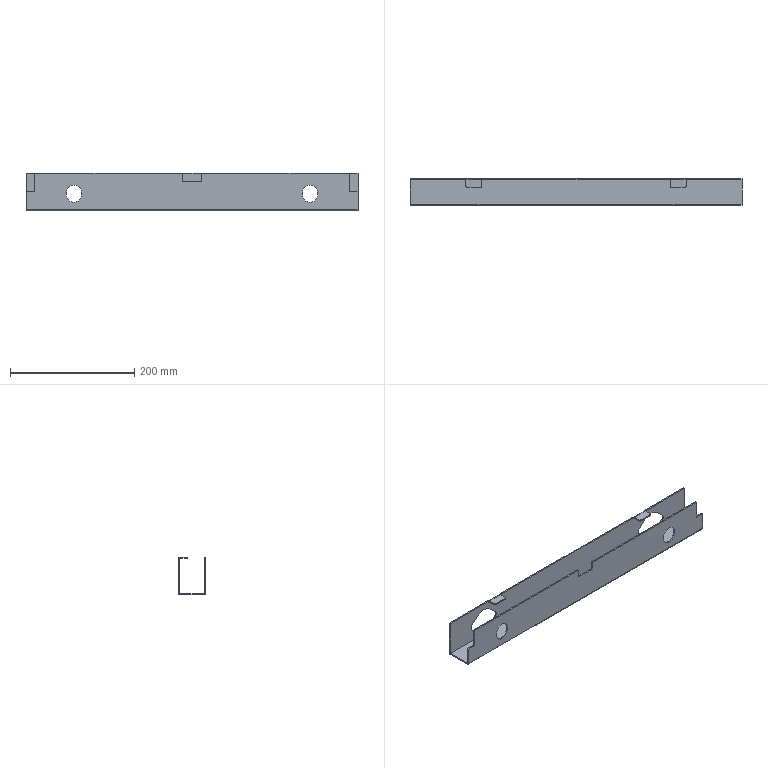Part | NX | features solid 2 | 1 solid | 88 faces | box 534 x 43.2 x 60.503 mm | volume 160058 mm3 | plane 58 | cylinder 26 | spline 4 | commonest cylinder face diameters 2 x4 6 x4 14 x4 24 x4 43 x4 0.4 x2